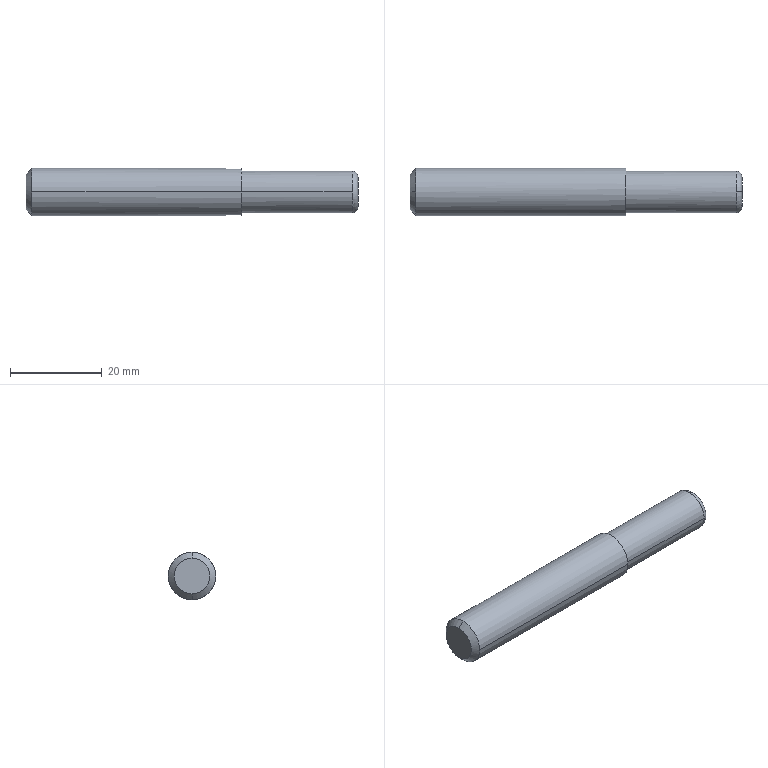Part | STEP file | 4-20.sldasm-Part-65 | 1 solid | 11 faces | box 72.39 x 10.317 x 10.317 mm | volume 5528 mm3 | cylinder 4 | plane 3 | torus 2 | cone 2 | commonest cylinder face diameters 9.047 x2 10.317 x2
STEP:
#1=CARTESIAN_POINT('',(264.37,-149.07,129.624));
#2=VERTEX_POINT('',#1);
#3=CARTESIAN_POINT('',(264.37,-144.546,125.1));
#4=VERTEX_POINT('',#3);
#5=CARTESIAN_POINT('',(264.37,-149.07,125.1));
#6=DIRECTION('',(-1.,0.,0.));
#7=DIRECTION('',(0.,0.,-1.));
#8=AXIS2_PLACEMENT_3D('',#5,#6,#7);
#9=CIRCLE('',#8,4.524);
#10=EDGE_CURVE('',#2,#4,#9,.T.);
#11=ORIENTED_EDGE('',*,*,#10,.F.);
#12=CARTESIAN_POINT('',(265.64,-149.07,128.354));
#13=VERTEX_POINT('',#12);
#14=CARTESIAN_POINT('',(264.37,-149.07,128.354));
#15=DIRECTION('',(0.,1.,0.));
#16=DIRECTION('',(0.,0.,1.));
#17=AXIS2_PLACEMENT_3D('',#14,#15,#16);
#18=CIRCLE('',#17,1.27);
#19=EDGE_CURVE('',#2,#13,#18,.T.);
#20=ORIENTED_EDGE('',*,*,#19,.T.);
#21=CARTESIAN_POINT('',(265.64,-149.07,121.846));
#22=VERTEX_POINT('',#21);
#23=CARTESIAN_POINT('',(265.64,-149.07,125.1));
#24=DIRECTION('',(1.,0.,0.));
#25=DIRECTION('',(0.,0.,-1.));
#26=AXIS2_PLACEMENT_3D('',#23,#24,#25);
#27=CIRCLE('',#26,3.254);
#28=EDGE_CURVE('',#22,#13,#27,.T.);
#29=ORIENTED_EDGE('',*,*,#28,.F.);
#30=CARTESIAN_POINT('',(264.37,-149.07,120.576));
#31=VERTEX_POINT('',#30);
#32=CARTESIAN_POINT('',(264.37,-149.07,121.846));
#33=DIRECTION('',(0.,-1.,0.));
#34=DIRECTION('',(0.,0.,-1.));
#35=AXIS2_PLACEMENT_3D('',#32,#33,#34);
#36=CIRCLE('',#35,1.27);
#37=EDGE_CURVE('',#31,#22,#36,.T.);
#38=ORIENTED_EDGE('',*,*,#37,.F.);
#39=CARTESIAN_POINT('',(264.37,-149.07,125.1));
#40=DIRECTION('',(-1.,0.,0.));
#41=DIRECTION('',(0.,0.,-1.));
#42=AXIS2_PLACEMENT_3D('',#39,#40,#41);
#43=CIRCLE('',#42,4.524);
#44=EDGE_CURVE('',#4,#31,#43,.T.);
#45=ORIENTED_EDGE('',*,*,#44,.F.);
#46=EDGE_LOOP('',(#11,#20,#29,#38,#45));
#47=FACE_OUTER_BOUND('',#46,.T.);
#48=CARTESIAN_POINT('',(264.37,-149.07,125.1));
#49=DIRECTION('',(1.,0.,0.));
#50=DIRECTION('',(0.,0.,-1.));
#51=AXIS2_PLACEMENT_3D('',#48,#49,#50);
#52=TOROIDAL_SURFACE('',#51,3.254,1.27);
#53=ADVANCED_FACE('',(#47),#52,.T.);
#54=CARTESIAN_POINT('',(264.37,-153.594,125.1));
#55=VERTEX_POINT('',#54);
#56=CARTESIAN_POINT('',(264.37,-149.07,125.1));
#57=DIRECTION('',(-1.,0.,0.));
#58=DIRECTION('',(0.,0.,-1.));
#59=AXIS2_PLACEMENT_3D('',#56,#57,#58);
#60=CIRCLE('',#59,4.524);
#61=EDGE_CURVE('',#55,#2,#60,.T.);
#62=ORIENTED_EDGE('',*,*,#61,.T.);
#63=ORIENTED_EDGE('',*,*,#10,.T.);
#64=CARTESIAN_POINT('',(240.24,-144.546,125.1));
#65=VERTEX_POINT('',#64);
#66=CARTESIAN_POINT('',(244.05,-144.546,125.1));
#67=DIRECTION('',(-1.,0.,0.));
#68=VECTOR('',#67,1000.);
#69=LINE('',#66,#68);
#70=EDGE_CURVE('',#4,#65,#69,.T.);
#71=ORIENTED_EDGE('',*,*,#70,.T.);
#72=CARTESIAN_POINT('',(240.24,-153.594,125.1));
#73=VERTEX_POINT('',#72);
#74=CARTESIAN_POINT('',(240.24,-149.07,125.1));
#75=DIRECTION('',(-1.,0.,0.));
#76=DIRECTION('',(0.,0.,-1.));
#77=AXIS2_PLACEMENT_3D('',#74,#75,#76);
#78=CIRCLE('',#77,4.524);
#79=EDGE_CURVE('',#73,#65,#78,.T.);
#80=ORIENTED_EDGE('',*,*,#79,.F.);
#81=CARTESIAN_POINT('',(244.05,-153.594,125.1));
#82=DIRECTION('',(-1.,0.,0.));
#83=VECTOR('',#82,1000.);
#84=LINE('',#81,#83);
#85=EDGE_CURVE('',#55,#73,#84,.T.);
#86=ORIENTED_EDGE('',*,*,#85,.F.);
#87=EDGE_LOOP('',(#62,#63,#71,#80,#86));
#88=FACE_OUTER_BOUND('',#87,.T.);
#89=CARTESIAN_POINT('',(244.05,-149.07,125.1));
#90=DIRECTION('',(-1.,0.,0.));
#91=DIRECTION('',(0.,-1.,0.));
#92=AXIS2_PLACEMENT_3D('',#89,#90,#91);
#93=CYLINDRICAL_SURFACE('',#92,4.524);
#94=ADVANCED_FACE('',(#88),#93,.T.);
#95=CARTESIAN_POINT('',(240.24,-154.229,125.1));
#96=VERTEX_POINT('',#95);
#97=CARTESIAN_POINT('',(240.24,-143.911,125.1));
#98=VERTEX_POINT('',#97);
#99=CARTESIAN_POINT('',(240.24,-149.07,125.1));
#100=DIRECTION('',(-1.,0.,0.));
#101=DIRECTION('',(0.,0.,-1.));
#102=AXIS2_PLACEMENT_3D('',#99,#100,#101);
#103=CIRCLE('',#102,5.159);
#104=EDGE_CURVE('',#96,#98,#103,.T.);
#105=ORIENTED_EDGE('',*,*,#104,.T.);
#106=CARTESIAN_POINT('',(194.52,-143.911,125.1));
#107=VERTEX_POINT('',#106);
#108=CARTESIAN_POINT('',(244.05,-143.911,125.1));
#109=DIRECTION('',(-1.,0.,0.));
#110=VECTOR('',#109,1000.);
#111=LINE('',#108,#110);
#112=EDGE_CURVE('',#98,#107,#111,.T.);
#113=ORIENTED_EDGE('',*,*,#112,.T.);
#114=CARTESIAN_POINT('',(194.52,-149.07,130.259));
#115=VERTEX_POINT('',#114);
#116=CARTESIAN_POINT('',(194.52,-149.07,125.1));
#117=DIRECTION('',(1.,0.,0.));
#118=DIRECTION('',(0.,0.,1.));
#119=AXIS2_PLACEMENT_3D('',#116,#117,#118);
#120=CIRCLE('',#119,5.159);
#121=EDGE_CURVE('',#107,#115,#120,.T.);
#122=ORIENTED_EDGE('',*,*,#121,.T.);
#123=CARTESIAN_POINT('',(194.52,-154.229,125.1));
#124=VERTEX_POINT('',#123);
#125=CARTESIAN_POINT('',(194.52,-149.07,125.1));
#126=DIRECTION('',(1.,0.,0.));
#127=DIRECTION('',(0.,0.,1.));
#128=AXIS2_PLACEMENT_3D('',#125,#126,#127);
#129=CIRCLE('',#128,5.159);
#130=EDGE_CURVE('',#115,#124,#129,.T.);
#131=ORIENTED_EDGE('',*,*,#130,.T.);
#132=CARTESIAN_POINT('',(244.05,-154.229,125.1));
#133=DIRECTION('',(-1.,0.,0.));
#134=VECTOR('',#133,1000.);
#135=LINE('',#132,#134);
#136=EDGE_CURVE('',#96,#124,#135,.T.);
#137=ORIENTED_EDGE('',*,*,#136,.F.);
#138=EDGE_LOOP('',(#105,#113,#122,#131,#137));
#139=FACE_OUTER_BOUND('',#138,.T.);
#140=CARTESIAN_POINT('',(244.05,-149.07,125.1));
#141=DIRECTION('',(-1.,0.,0.));
#142=DIRECTION('',(0.,-1.,0.));
#143=AXIS2_PLACEMENT_3D('',#140,#141,#142);
#144=CYLINDRICAL_SURFACE('',#143,5.159);
#145=ADVANCED_FACE('',(#139),#144,.T.);
#146=CARTESIAN_POINT('',(193.25,-149.07,128.989));
#147=VERTEX_POINT('',#146);
#148=CARTESIAN_POINT('',(193.25,-149.07,121.211));
#149=VERTEX_POINT('',#148);
#150=CARTESIAN_POINT('',(193.25,-149.07,125.1));
#151=DIRECTION('',(-1.,0.,0.));
#152=DIRECTION('',(0.,0.,1.));
#153=AXIS2_PLACEMENT_3D('',#150,#151,#152);
#154=CIRCLE('',#153,3.889);
#155=EDGE_CURVE('',#147,#149,#154,.T.);
#156=ORIENTED_EDGE('',*,*,#155,.F.);
#157=CARTESIAN_POINT('',(193.25,-149.07,128.989));
#158=DIRECTION('',(0.7071,0.,0.7071));
#159=VECTOR('',#158,1000.);
#160=LINE('',#157,#159);
#161=EDGE_CURVE('',#147,#115,#160,.T.);
#162=ORIENTED_EDGE('',*,*,#161,.T.);
#163=ORIENTED_EDGE('',*,*,#121,.F.);
#164=CARTESIAN_POINT('',(194.52,-149.07,119.941));
#165=VERTEX_POINT('',#164);
#166=CARTESIAN_POINT('',(194.52,-149.07,125.1));
#167=DIRECTION('',(1.,0.,0.));
#168=DIRECTION('',(0.,0.,1.));
#169=AXIS2_PLACEMENT_3D('',#166,#167,#168);
#170=CIRCLE('',#169,5.159);
#171=EDGE_CURVE('',#165,#107,#170,.T.);
#172=ORIENTED_EDGE('',*,*,#171,.F.);
#173=CARTESIAN_POINT('',(193.25,-149.07,121.211));
#174=DIRECTION('',(0.7071,0.,-0.7071));
#175=VECTOR('',#174,1000.);
#176=LINE('',#173,#175);
#177=EDGE_CURVE('',#149,#165,#176,.T.);
#178=ORIENTED_EDGE('',*,*,#177,.F.);
#179=EDGE_LOOP('',(#156,#162,#163,#172,#178));
#180=FACE_OUTER_BOUND('',#179,.T.);
#181=CARTESIAN_POINT('',(193.25,-149.07,125.1));
#182=DIRECTION('',(1.,0.,0.));
#183=DIRECTION('',(0.,0.,-1.));
#184=AXIS2_PLACEMENT_3D('',#181,#182,#183);
#185=CONICAL_SURFACE('',#184,3.889,0.7854);
#186=ADVANCED_FACE('',(#180),#185,.T.);
#187=ORIENTED_EDGE('',*,*,#104,.F.);
#188=CARTESIAN_POINT('',(240.24,-149.07,125.1));
#189=DIRECTION('',(-1.,0.,0.));
#190=DIRECTION('',(0.,0.,-1.));
#191=AXIS2_PLACEMENT_3D('',#188,#189,#190);
#192=CIRCLE('',#191,5.159);
#193=EDGE_CURVE('',#98,#96,#192,.T.);
#194=ORIENTED_EDGE('',*,*,#193,.F.);
#195=EDGE_LOOP('',(#187,#194));
#196=FACE_OUTER_BOUND('',#195,.T.);
#197=ORIENTED_EDGE('',*,*,#79,.T.);
#198=CARTESIAN_POINT('',(240.24,-149.07,125.1));
#199=DIRECTION('',(-1.,0.,0.));
#200=DIRECTION('',(0.,0.,-1.));
#201=AXIS2_PLACEMENT_3D('',#198,#199,#200);
#202=CIRCLE('',#201,4.524);
#203=EDGE_CURVE('',#65,#73,#202,.T.);
#204=ORIENTED_EDGE('',*,*,#203,.T.);
#205=EDGE_LOOP('',(#197,#204));
#206=FACE_BOUND('',#205,.T.);
#207=CARTESIAN_POINT('',(240.24,-149.07,125.1));
#208=DIRECTION('',(1.,0.,0.));
#209=DIRECTION('',(0.,0.,-1.));
#210=AXIS2_PLACEMENT_3D('',#207,#208,#209);
#211=PLANE('',#210);
#212=ADVANCED_FACE('',(#196,#206),#211,.T.);
#213=CARTESIAN_POINT('',(193.25,-149.07,125.1));
#214=DIRECTION('',(-1.,0.,0.));
#215=DIRECTION('',(0.,0.,1.));
#216=AXIS2_PLACEMENT_3D('',#213,#214,#215);
#217=CIRCLE('',#216,3.889);
#218=EDGE_CURVE('',#149,#147,#217,.T.);
#219=ORIENTED_EDGE('',*,*,#218,.T.);
#220=ORIENTED_EDGE('',*,*,#155,.T.);
#221=EDGE_LOOP('',(#219,#220));
#222=FACE_OUTER_BOUND('',#221,.T.);
#223=CARTESIAN_POINT('',(193.25,-149.07,125.1));
#224=DIRECTION('',(-1.,0.,0.));
#225=DIRECTION('',(0.,-1.,0.));
#226=AXIS2_PLACEMENT_3D('',#223,#224,#225);
#227=PLANE('',#226);
#228=ADVANCED_FACE('',(#222),#227,.T.);
#229=ORIENTED_EDGE('',*,*,#161,.F.);
#230=ORIENTED_EDGE('',*,*,#218,.F.);
#231=ORIENTED_EDGE('',*,*,#177,.T.);
#232=CARTESIAN_POINT('',(194.52,-149.07,125.1));
#233=DIRECTION('',(1.,0.,0.));
#234=DIRECTION('',(0.,0.,1.));
#235=AXIS2_PLACEMENT_3D('',#232,#233,#234);
#236=CIRCLE('',#235,5.159);
#237=EDGE_CURVE('',#124,#165,#236,.T.);
#238=ORIENTED_EDGE('',*,*,#237,.F.);
#239=ORIENTED_EDGE('',*,*,#130,.F.);
#240=EDGE_LOOP('',(#229,#230,#231,#238,#239));
#241=FACE_OUTER_BOUND('',#240,.T.);
#242=CARTESIAN_POINT('',(193.25,-149.07,125.1));
#243=DIRECTION('',(1.,0.,0.));
#244=DIRECTION('',(0.,0.,-1.));
#245=AXIS2_PLACEMENT_3D('',#242,#243,#244);
#246=CONICAL_SURFACE('',#245,3.889,0.7854);
#247=ADVANCED_FACE('',(#241),#246,.T.);
#248=ORIENTED_EDGE('',*,*,#112,.F.);
#249=ORIENTED_EDGE('',*,*,#193,.T.);
#250=ORIENTED_EDGE('',*,*,#136,.T.);
#251=ORIENTED_EDGE('',*,*,#237,.T.);
#252=ORIENTED_EDGE('',*,*,#171,.T.);
#253=EDGE_LOOP('',(#248,#249,#250,#251,#252));
#254=FACE_OUTER_BOUND('',#253,.T.);
#255=CARTESIAN_POINT('',(244.05,-149.07,125.1));
#256=DIRECTION('',(-1.,0.,0.));
#257=DIRECTION('',(0.,-1.,0.));
#258=AXIS2_PLACEMENT_3D('',#255,#256,#257);
#259=CYLINDRICAL_SURFACE('',#258,5.159);
#260=ADVANCED_FACE('',(#254),#259,.T.);
#261=ORIENTED_EDGE('',*,*,#70,.F.);
#262=ORIENTED_EDGE('',*,*,#44,.T.);
#263=CARTESIAN_POINT('',(264.37,-149.07,125.1));
#264=DIRECTION('',(-1.,0.,0.));
#265=DIRECTION('',(0.,0.,-1.));
#266=AXIS2_PLACEMENT_3D('',#263,#264,#265);
#267=CIRCLE('',#266,4.524);
#268=EDGE_CURVE('',#31,#55,#267,.T.);
#269=ORIENTED_EDGE('',*,*,#268,.T.);
#270=ORIENTED_EDGE('',*,*,#85,.T.);
#271=ORIENTED_EDGE('',*,*,#203,.F.);
#272=EDGE_LOOP('',(#261,#262,#269,#270,#271));
#273=FACE_OUTER_BOUND('',#272,.T.);
#274=CARTESIAN_POINT('',(244.05,-149.07,125.1));
#275=DIRECTION('',(-1.,0.,0.));
#276=DIRECTION('',(0.,-1.,0.));
#277=AXIS2_PLACEMENT_3D('',#274,#275,#276);
#278=CYLINDRICAL_SURFACE('',#277,4.524);
#279=ADVANCED_FACE('',(#273),#278,.T.);
#280=ORIENTED_EDGE('',*,*,#28,.T.);
#281=CARTESIAN_POINT('',(265.64,-149.07,125.1));
#282=DIRECTION('',(1.,0.,0.));
#283=DIRECTION('',(0.,0.,-1.));
#284=AXIS2_PLACEMENT_3D('',#281,#282,#283);
#285=CIRCLE('',#284,3.254);
#286=EDGE_CURVE('',#13,#22,#285,.T.);
#287=ORIENTED_EDGE('',*,*,#286,.T.);
#288=EDGE_LOOP('',(#280,#287));
#289=FACE_OUTER_BOUND('',#288,.T.);
#290=CARTESIAN_POINT('',(265.64,-149.07,125.1));
#291=DIRECTION('',(1.,0.,0.));
#292=DIRECTION('',(0.,0.,-1.));
#293=AXIS2_PLACEMENT_3D('',#290,#291,#292);
#294=PLANE('',#293);
#295=ADVANCED_FACE('',(#289),#294,.T.);
#296=ORIENTED_EDGE('',*,*,#19,.F.);
#297=ORIENTED_EDGE('',*,*,#61,.F.);
#298=ORIENTED_EDGE('',*,*,#268,.F.);
#299=ORIENTED_EDGE('',*,*,#37,.T.);
#300=ORIENTED_EDGE('',*,*,#286,.F.);
#301=EDGE_LOOP('',(#296,#297,#298,#299,#300));
#302=FACE_OUTER_BOUND('',#301,.T.);
#303=CARTESIAN_POINT('',(264.37,-149.07,125.1));
#304=DIRECTION('',(1.,0.,0.));
#305=DIRECTION('',(0.,0.,-1.));
#306=AXIS2_PLACEMENT_3D('',#303,#304,#305);
#307=TOROIDAL_SURFACE('',#306,3.254,1.27);
#308=ADVANCED_FACE('',(#302),#307,.T.);
#309=CLOSED_SHELL('',(#53,#94,#145,#186,#212,#228,#247,#260,#279,#295,#308));
#310=MANIFOLD_SOLID_BREP('',#309);
#311=CARTESIAN_POINT('',(0.,0.,0.));
#312=DIRECTION('',(0.,0.,1.));
#313=DIRECTION('',(1.,0.,0.));
#314=AXIS2_PLACEMENT_3D('',#311,#312,#313);
#315=(LENGTH_UNIT()NAMED_UNIT(*)SI_UNIT(.MILLI.,.METRE.));
#316=UNCERTAINTY_MEASURE_WITH_UNIT(LENGTH_MEASURE(0.00001),#315,'','');
#317=(NAMED_UNIT(*)PLANE_ANGLE_UNIT()SI_UNIT($,.RADIAN.));
#318=(NAMED_UNIT(*)SI_UNIT($,.STERADIAN.)SOLID_ANGLE_UNIT());
#319=(GEOMETRIC_REPRESENTATION_CONTEXT(3)GLOBAL_UNCERTAINTY_ASSIGNED_CONTEXT((#316))GLOBAL_UNIT_ASSIGNED_CONTEXT((#315,#317,#318))REPRESENTATION_CONTEXT('',''));
#320=ADVANCED_BREP_SHAPE_REPRESENTATION('',(#310,#314),#319);